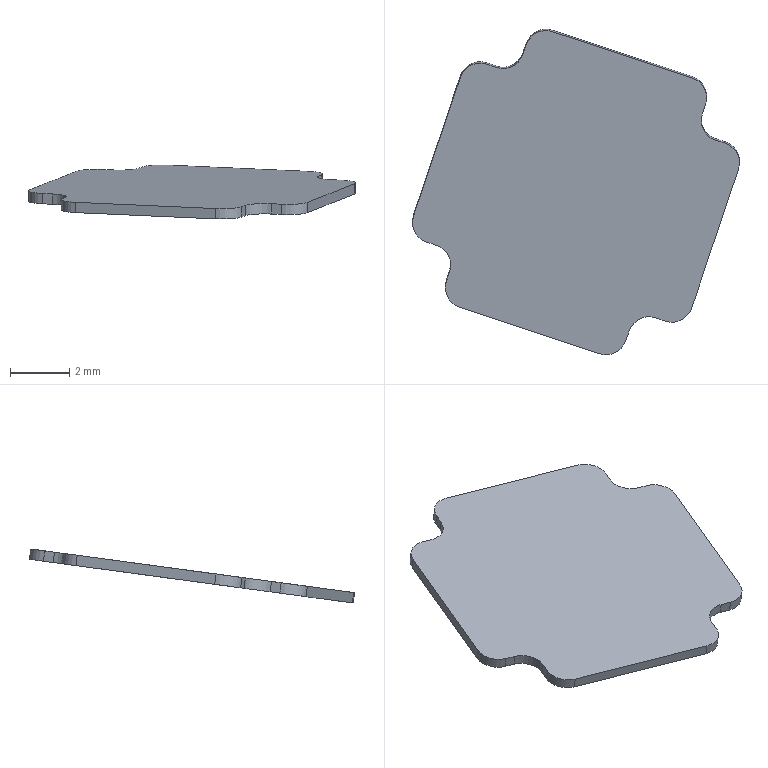Part | SolidWorks | features SplitBody 1 | 1 solid | 26 faces | box 11.072 x 11.019 x 1.829 mm | volume 30.173 mm3 | plane 14 | cylinder 12 | commonest cylinder face diameters 1.408 x12
STEP:
#1=CARTESIAN_POINT('',(543.22,367.896,-325.051));
#2=VERTEX_POINT('',#1);
#3=CARTESIAN_POINT('',(542.329,367.455,-325.11));
#4=VERTEX_POINT('',#3);
#5=CARTESIAN_POINT('',(542.997,367.234,-325.14));
#6=DIRECTION('',(0.,-0.1337,0.991));
#7=DIRECTION('',(0.317,0.9399,0.1268));
#8=AXIS2_PLACEMENT_3D('',#5,#6,#7);
#9=CIRCLE('',#8,0.704);
#10=EDGE_CURVE('',#2,#4,#9,.T.);
#11=ORIENTED_EDGE('',*,*,#10,.T.);
#12=CARTESIAN_POINT('',(542.329,367.408,-324.761));
#13=VERTEX_POINT('',#12);
#14=CARTESIAN_POINT('',(542.329,367.408,-324.761));
#15=DIRECTION('',(0.,0.1337,-0.991));
#16=VECTOR('',#15,1000.);
#17=LINE('',#14,#16);
#18=EDGE_CURVE('',#13,#4,#17,.T.);
#19=ORIENTED_EDGE('',*,*,#18,.F.);
#20=CARTESIAN_POINT('',(543.22,367.849,-324.702));
#21=VERTEX_POINT('',#20);
#22=CARTESIAN_POINT('',(542.997,367.187,-324.791));
#23=DIRECTION('',(0.,-0.1337,0.991));
#24=DIRECTION('',(0.317,0.9399,0.1268));
#25=AXIS2_PLACEMENT_3D('',#22,#23,#24);
#26=CIRCLE('',#25,0.704);
#27=EDGE_CURVE('',#21,#13,#26,.T.);
#28=ORIENTED_EDGE('',*,*,#27,.F.);
#29=CARTESIAN_POINT('',(543.22,367.849,-324.702));
#30=DIRECTION('',(0.,0.1337,-0.991));
#31=VECTOR('',#30,1000.);
#32=LINE('',#29,#31);
#33=EDGE_CURVE('',#21,#2,#32,.T.);
#34=ORIENTED_EDGE('',*,*,#33,.T.);
#35=EDGE_LOOP('',(#11,#19,#28,#34));
#36=FACE_OUTER_BOUND('',#35,.T.);
#37=CARTESIAN_POINT('',(542.997,367.187,-324.791));
#38=DIRECTION('',(0.,0.1337,-0.991));
#39=DIRECTION('',(0.317,0.9399,0.1268));
#40=AXIS2_PLACEMENT_3D('',#37,#38,#39);
#41=CYLINDRICAL_SURFACE('',#40,0.704);
#42=ADVANCED_FACE('',(#36),#41,.T.);
#43=CARTESIAN_POINT('',(542.217,367.125,-325.155));
#44=VERTEX_POINT('',#43);
#45=CARTESIAN_POINT('',(542.329,367.455,-325.11));
#46=DIRECTION('',(-0.317,-0.9399,-0.1268));
#47=VECTOR('',#46,1000.);
#48=LINE('',#45,#47);
#49=EDGE_CURVE('',#4,#44,#48,.T.);
#50=ORIENTED_EDGE('',*,*,#49,.T.);
#51=CARTESIAN_POINT('',(542.217,367.078,-324.806));
#52=VERTEX_POINT('',#51);
#53=CARTESIAN_POINT('',(542.217,367.078,-324.806));
#54=DIRECTION('',(0.,0.1337,-0.991));
#55=VECTOR('',#54,1000.);
#56=LINE('',#53,#55);
#57=EDGE_CURVE('',#52,#44,#56,.T.);
#58=ORIENTED_EDGE('',*,*,#57,.F.);
#59=CARTESIAN_POINT('',(542.329,367.408,-324.761));
#60=DIRECTION('',(-0.317,-0.9399,-0.1268));
#61=VECTOR('',#60,1000.);
#62=LINE('',#59,#61);
#63=EDGE_CURVE('',#13,#52,#62,.T.);
#64=ORIENTED_EDGE('',*,*,#63,.F.);
#65=ORIENTED_EDGE('',*,*,#18,.T.);
#66=EDGE_LOOP('',(#50,#58,#64,#65));
#67=FACE_OUTER_BOUND('',#66,.T.);
#68=CARTESIAN_POINT('',(542.329,367.408,-324.761));
#69=DIRECTION('',(0.9484,-0.3142,-0.04237));
#70=DIRECTION('',(0.,-0.1337,0.991));
#71=AXIS2_PLACEMENT_3D('',#68,#69,#70);
#72=PLANE('',#71);
#73=ADVANCED_FACE('',(#67),#72,.F.);
#74=CARTESIAN_POINT('',(541.326,366.684,-325.214));
#75=VERTEX_POINT('',#74);
#76=CARTESIAN_POINT('',(541.55,367.346,-325.125));
#77=DIRECTION('',(0.,0.1337,-0.991));
#78=DIRECTION('',(0.317,0.9399,0.1268));
#79=AXIS2_PLACEMENT_3D('',#76,#77,#78);
#80=CIRCLE('',#79,0.704);
#81=EDGE_CURVE('',#44,#75,#80,.T.);
#82=ORIENTED_EDGE('',*,*,#81,.T.);
#83=CARTESIAN_POINT('',(541.326,366.637,-324.865));
#84=VERTEX_POINT('',#83);
#85=CARTESIAN_POINT('',(541.326,366.637,-324.865));
#86=DIRECTION('',(0.,0.1337,-0.991));
#87=VECTOR('',#86,1000.);
#88=LINE('',#85,#87);
#89=EDGE_CURVE('',#84,#75,#88,.T.);
#90=ORIENTED_EDGE('',*,*,#89,.F.);
#91=CARTESIAN_POINT('',(541.55,367.299,-324.776));
#92=DIRECTION('',(0.,0.1337,-0.991));
#93=DIRECTION('',(0.317,0.9399,0.1268));
#94=AXIS2_PLACEMENT_3D('',#91,#92,#93);
#95=CIRCLE('',#94,0.704);
#96=EDGE_CURVE('',#52,#84,#95,.T.);
#97=ORIENTED_EDGE('',*,*,#96,.F.);
#98=ORIENTED_EDGE('',*,*,#57,.T.);
#99=EDGE_LOOP('',(#82,#90,#97,#98));
#100=FACE_OUTER_BOUND('',#99,.T.);
#101=CARTESIAN_POINT('',(541.55,367.299,-324.776));
#102=DIRECTION('',(0.,0.1337,-0.991));
#103=DIRECTION('',(0.317,0.9399,0.1268));
#104=AXIS2_PLACEMENT_3D('',#101,#102,#103);
#105=CYLINDRICAL_SURFACE('',#104,0.704);
#106=ADVANCED_FACE('',(#100),#105,.F.);
#107=CARTESIAN_POINT('',(540.993,366.795,-325.199));
#108=VERTEX_POINT('',#107);
#109=CARTESIAN_POINT('',(541.326,366.684,-325.214));
#110=DIRECTION('',(-0.9484,0.3142,0.04237));
#111=VECTOR('',#110,1000.);
#112=LINE('',#109,#111);
#113=EDGE_CURVE('',#75,#108,#112,.T.);
#114=ORIENTED_EDGE('',*,*,#113,.T.);
#115=CARTESIAN_POINT('',(540.993,366.748,-324.85));
#116=VERTEX_POINT('',#115);
#117=CARTESIAN_POINT('',(540.993,366.748,-324.85));
#118=DIRECTION('',(0.,0.1337,-0.991));
#119=VECTOR('',#118,1000.);
#120=LINE('',#117,#119);
#121=EDGE_CURVE('',#116,#108,#120,.T.);
#122=ORIENTED_EDGE('',*,*,#121,.F.);
#123=CARTESIAN_POINT('',(541.326,366.637,-324.865));
#124=DIRECTION('',(-0.9484,0.3142,0.04237));
#125=VECTOR('',#124,1000.);
#126=LINE('',#123,#125);
#127=EDGE_CURVE('',#84,#116,#126,.T.);
#128=ORIENTED_EDGE('',*,*,#127,.F.);
#129=ORIENTED_EDGE('',*,*,#89,.T.);
#130=EDGE_LOOP('',(#114,#122,#128,#129));
#131=FACE_OUTER_BOUND('',#130,.T.);
#132=CARTESIAN_POINT('',(541.326,366.637,-324.865));
#133=DIRECTION('',(-0.317,-0.9399,-0.1268));
#134=DIRECTION('',(0.,0.1337,-0.991));
#135=AXIS2_PLACEMENT_3D('',#132,#133,#134);
#136=PLANE('',#135);
#137=ADVANCED_FACE('',(#131),#136,.F.);
#138=CARTESIAN_POINT('',(540.102,366.354,-325.259));
#139=VERTEX_POINT('',#138);
#140=CARTESIAN_POINT('',(540.769,366.133,-325.288));
#141=DIRECTION('',(0.,-0.1337,0.991));
#142=DIRECTION('',(-0.317,-0.9399,-0.1268));
#143=AXIS2_PLACEMENT_3D('',#140,#141,#142);
#144=CIRCLE('',#143,0.704);
#145=EDGE_CURVE('',#108,#139,#144,.T.);
#146=ORIENTED_EDGE('',*,*,#145,.T.);
#147=CARTESIAN_POINT('',(540.102,366.307,-324.91));
#148=VERTEX_POINT('',#147);
#149=CARTESIAN_POINT('',(540.102,366.307,-324.91));
#150=DIRECTION('',(0.,0.1337,-0.991));
#151=VECTOR('',#150,1000.);
#152=LINE('',#149,#151);
#153=EDGE_CURVE('',#148,#139,#152,.T.);
#154=ORIENTED_EDGE('',*,*,#153,.F.);
#155=CARTESIAN_POINT('',(540.769,366.086,-324.94));
#156=DIRECTION('',(0.,-0.1337,0.991));
#157=DIRECTION('',(-0.317,-0.9399,-0.1268));
#158=AXIS2_PLACEMENT_3D('',#155,#156,#157);
#159=CIRCLE('',#158,0.704);
#160=EDGE_CURVE('',#116,#148,#159,.T.);
#161=ORIENTED_EDGE('',*,*,#160,.F.);
#162=ORIENTED_EDGE('',*,*,#121,.T.);
#163=EDGE_LOOP('',(#146,#154,#161,#162));
#164=FACE_OUTER_BOUND('',#163,.T.);
#165=CARTESIAN_POINT('',(540.769,366.086,-324.94));
#166=DIRECTION('',(0.,0.1337,-0.991));
#167=DIRECTION('',(0.317,0.9399,0.1268));
#168=AXIS2_PLACEMENT_3D('',#165,#166,#167);
#169=CYLINDRICAL_SURFACE('',#168,0.704);
#170=ADVANCED_FACE('',(#164),#169,.T.);
#171=CARTESIAN_POINT('',(538.517,361.656,-325.892));
#172=VERTEX_POINT('',#171);
#173=CARTESIAN_POINT('',(540.102,366.354,-325.259));
#174=DIRECTION('',(-0.317,-0.9399,-0.1268));
#175=VECTOR('',#174,1000.);
#176=LINE('',#173,#175);
#177=EDGE_CURVE('',#139,#172,#176,.T.);
#178=ORIENTED_EDGE('',*,*,#177,.T.);
#179=CARTESIAN_POINT('',(538.517,361.609,-325.543));
#180=VERTEX_POINT('',#179);
#181=CARTESIAN_POINT('',(538.517,361.609,-325.543));
#182=DIRECTION('',(0.,0.1337,-0.991));
#183=VECTOR('',#182,1000.);
#184=LINE('',#181,#183);
#185=EDGE_CURVE('',#180,#172,#184,.T.);
#186=ORIENTED_EDGE('',*,*,#185,.F.);
#187=CARTESIAN_POINT('',(540.102,366.307,-324.91));
#188=DIRECTION('',(-0.317,-0.9399,-0.1268));
#189=VECTOR('',#188,1000.);
#190=LINE('',#187,#189);
#191=EDGE_CURVE('',#148,#180,#190,.T.);
#192=ORIENTED_EDGE('',*,*,#191,.F.);
#193=ORIENTED_EDGE('',*,*,#153,.T.);
#194=EDGE_LOOP('',(#178,#186,#192,#193));
#195=FACE_OUTER_BOUND('',#194,.T.);
#196=CARTESIAN_POINT('',(540.102,366.307,-324.91));
#197=DIRECTION('',(0.9484,-0.3142,-0.04237));
#198=DIRECTION('',(0.,-0.1337,0.991));
#199=AXIS2_PLACEMENT_3D('',#196,#197,#198);
#200=PLANE('',#199);
#201=ADVANCED_FACE('',(#195),#200,.F.);
#202=CARTESIAN_POINT('',(538.962,360.773,-326.011));
#203=VERTEX_POINT('',#202);
#204=CARTESIAN_POINT('',(539.185,361.435,-325.922));
#205=DIRECTION('',(0.,-0.1337,0.991));
#206=DIRECTION('',(0.317,0.9399,0.1268));
#207=AXIS2_PLACEMENT_3D('',#204,#205,#206);
#208=CIRCLE('',#207,0.704);
#209=EDGE_CURVE('',#172,#203,#208,.T.);
#210=ORIENTED_EDGE('',*,*,#209,.T.);
#211=CARTESIAN_POINT('',(538.962,360.726,-325.662));
#212=VERTEX_POINT('',#211);
#213=CARTESIAN_POINT('',(538.962,360.726,-325.662));
#214=DIRECTION('',(0.,0.1337,-0.991));
#215=VECTOR('',#214,1000.);
#216=LINE('',#213,#215);
#217=EDGE_CURVE('',#212,#203,#216,.T.);
#218=ORIENTED_EDGE('',*,*,#217,.F.);
#219=CARTESIAN_POINT('',(539.185,361.388,-325.573));
#220=DIRECTION('',(0.,-0.1337,0.991));
#221=DIRECTION('',(0.317,0.9399,0.1268));
#222=AXIS2_PLACEMENT_3D('',#219,#220,#221);
#223=CIRCLE('',#222,0.704);
#224=EDGE_CURVE('',#180,#212,#223,.T.);
#225=ORIENTED_EDGE('',*,*,#224,.F.);
#226=ORIENTED_EDGE('',*,*,#185,.T.);
#227=EDGE_LOOP('',(#210,#218,#225,#226));
#228=FACE_OUTER_BOUND('',#227,.T.);
#229=CARTESIAN_POINT('',(539.185,361.388,-325.573));
#230=DIRECTION('',(0.,0.1337,-0.991));
#231=DIRECTION('',(0.317,0.9399,0.1268));
#232=AXIS2_PLACEMENT_3D('',#229,#230,#231);
#233=CYLINDRICAL_SURFACE('',#232,0.704);
#234=ADVANCED_FACE('',(#228),#233,.T.);
#235=CARTESIAN_POINT('',(539.296,360.663,-326.026));
#236=VERTEX_POINT('',#235);
#237=CARTESIAN_POINT('',(538.962,360.773,-326.011));
#238=DIRECTION('',(0.9484,-0.3142,-0.04237));
#239=VECTOR('',#238,1000.);
#240=LINE('',#237,#239);
#241=EDGE_CURVE('',#203,#236,#240,.T.);
#242=ORIENTED_EDGE('',*,*,#241,.T.);
#243=CARTESIAN_POINT('',(539.296,360.616,-325.677));
#244=VERTEX_POINT('',#243);
#245=CARTESIAN_POINT('',(539.296,360.616,-325.677));
#246=DIRECTION('',(0.,0.1337,-0.991));
#247=VECTOR('',#246,1000.);
#248=LINE('',#245,#247);
#249=EDGE_CURVE('',#244,#236,#248,.T.);
#250=ORIENTED_EDGE('',*,*,#249,.F.);
#251=CARTESIAN_POINT('',(538.962,360.726,-325.662));
#252=DIRECTION('',(0.9484,-0.3142,-0.04237));
#253=VECTOR('',#252,1000.);
#254=LINE('',#251,#253);
#255=EDGE_CURVE('',#212,#244,#254,.T.);
#256=ORIENTED_EDGE('',*,*,#255,.F.);
#257=ORIENTED_EDGE('',*,*,#217,.T.);
#258=EDGE_LOOP('',(#242,#250,#256,#257));
#259=FACE_OUTER_BOUND('',#258,.T.);
#260=CARTESIAN_POINT('',(538.962,360.726,-325.662));
#261=DIRECTION('',(0.317,0.9399,0.1268));
#262=DIRECTION('',(0.,-0.1337,0.991));
#263=AXIS2_PLACEMENT_3D('',#260,#261,#262);
#264=PLANE('',#263);
#265=ADVANCED_FACE('',(#259),#264,.F.);
#266=CARTESIAN_POINT('',(539.74,359.78,-326.145));
#267=VERTEX_POINT('',#266);
#268=CARTESIAN_POINT('',(539.072,360.001,-326.115));
#269=DIRECTION('',(0.,0.1337,-0.991));
#270=DIRECTION('',(0.317,0.9399,0.1268));
#271=AXIS2_PLACEMENT_3D('',#268,#269,#270);
#272=CIRCLE('',#271,0.704);
#273=EDGE_CURVE('',#236,#267,#272,.T.);
#274=ORIENTED_EDGE('',*,*,#273,.T.);
#275=CARTESIAN_POINT('',(539.74,359.733,-325.796));
#276=VERTEX_POINT('',#275);
#277=CARTESIAN_POINT('',(539.74,359.733,-325.796));
#278=DIRECTION('',(0.,0.1337,-0.991));
#279=VECTOR('',#278,1000.);
#280=LINE('',#277,#279);
#281=EDGE_CURVE('',#276,#267,#280,.T.);
#282=ORIENTED_EDGE('',*,*,#281,.F.);
#283=CARTESIAN_POINT('',(539.072,359.954,-325.767));
#284=DIRECTION('',(0.,0.1337,-0.991));
#285=DIRECTION('',(0.317,0.9399,0.1268));
#286=AXIS2_PLACEMENT_3D('',#283,#284,#285);
#287=CIRCLE('',#286,0.704);
#288=EDGE_CURVE('',#244,#276,#287,.T.);
#289=ORIENTED_EDGE('',*,*,#288,.F.);
#290=ORIENTED_EDGE('',*,*,#249,.T.);
#291=EDGE_LOOP('',(#274,#282,#289,#290));
#292=FACE_OUTER_BOUND('',#291,.T.);
#293=CARTESIAN_POINT('',(539.072,359.954,-325.767));
#294=DIRECTION('',(0.,0.1337,-0.991));
#295=DIRECTION('',(0.317,0.9399,0.1268));
#296=AXIS2_PLACEMENT_3D('',#293,#294,#295);
#297=CYLINDRICAL_SURFACE('',#296,0.704);
#298=ADVANCED_FACE('',(#292),#297,.F.);
#299=CARTESIAN_POINT('',(539.628,359.449,-326.19));
#300=VERTEX_POINT('',#299);
#301=CARTESIAN_POINT('',(539.74,359.78,-326.145));
#302=DIRECTION('',(-0.317,-0.9399,-0.1268));
#303=VECTOR('',#302,1000.);
#304=LINE('',#301,#303);
#305=EDGE_CURVE('',#267,#300,#304,.T.);
#306=ORIENTED_EDGE('',*,*,#305,.T.);
#307=CARTESIAN_POINT('',(539.628,359.402,-325.841));
#308=VERTEX_POINT('',#307);
#309=CARTESIAN_POINT('',(539.628,359.402,-325.841));
#310=DIRECTION('',(0.,0.1337,-0.991));
#311=VECTOR('',#310,1000.);
#312=LINE('',#309,#311);
#313=EDGE_CURVE('',#308,#300,#312,.T.);
#314=ORIENTED_EDGE('',*,*,#313,.F.);
#315=CARTESIAN_POINT('',(539.74,359.733,-325.796));
#316=DIRECTION('',(-0.317,-0.9399,-0.1268));
#317=VECTOR('',#316,1000.);
#318=LINE('',#315,#317);
#319=EDGE_CURVE('',#276,#308,#318,.T.);
#320=ORIENTED_EDGE('',*,*,#319,.F.);
#321=ORIENTED_EDGE('',*,*,#281,.T.);
#322=EDGE_LOOP('',(#306,#314,#320,#321));
#323=FACE_OUTER_BOUND('',#322,.T.);
#324=CARTESIAN_POINT('',(539.74,359.733,-325.796));
#325=DIRECTION('',(0.9484,-0.3142,-0.04237));
#326=DIRECTION('',(0.,-0.1337,0.991));
#327=AXIS2_PLACEMENT_3D('',#324,#325,#326);
#328=PLANE('',#327);
#329=ADVANCED_FACE('',(#323),#328,.F.);
#330=CARTESIAN_POINT('',(540.073,358.566,-326.309));
#331=VERTEX_POINT('',#330);
#332=CARTESIAN_POINT('',(540.296,359.228,-326.22));
#333=DIRECTION('',(0.,-0.1337,0.991));
#334=DIRECTION('',(-0.317,-0.9399,-0.1268));
#335=AXIS2_PLACEMENT_3D('',#332,#333,#334);
#336=CIRCLE('',#335,0.704);
#337=EDGE_CURVE('',#300,#331,#336,.T.);
#338=ORIENTED_EDGE('',*,*,#337,.T.);
#339=CARTESIAN_POINT('',(540.073,358.519,-325.96));
#340=VERTEX_POINT('',#339);
#341=CARTESIAN_POINT('',(540.073,358.519,-325.96));
#342=DIRECTION('',(0.,0.1337,-0.991));
#343=VECTOR('',#342,1000.);
#344=LINE('',#341,#343);
#345=EDGE_CURVE('',#340,#331,#344,.T.);
#346=ORIENTED_EDGE('',*,*,#345,.F.);
#347=CARTESIAN_POINT('',(540.296,359.181,-325.871));
#348=DIRECTION('',(0.,-0.1337,0.991));
#349=DIRECTION('',(-0.317,-0.9399,-0.1268));
#350=AXIS2_PLACEMENT_3D('',#347,#348,#349);
#351=CIRCLE('',#350,0.704);
#352=EDGE_CURVE('',#308,#340,#351,.T.);
#353=ORIENTED_EDGE('',*,*,#352,.F.);
#354=ORIENTED_EDGE('',*,*,#313,.T.);
#355=EDGE_LOOP('',(#338,#346,#353,#354));
#356=FACE_OUTER_BOUND('',#355,.T.);
#357=CARTESIAN_POINT('',(540.296,359.181,-325.871));
#358=DIRECTION('',(0.,0.1337,-0.991));
#359=DIRECTION('',(0.317,0.9399,0.1268));
#360=AXIS2_PLACEMENT_3D('',#357,#358,#359);
#361=CYLINDRICAL_SURFACE('',#360,0.704);
#362=ADVANCED_FACE('',(#356),#361,.T.);
#363=CARTESIAN_POINT('',(544.814,356.996,-326.521));
#364=VERTEX_POINT('',#363);
#365=CARTESIAN_POINT('',(540.073,358.566,-326.309));
#366=DIRECTION('',(0.9484,-0.3142,-0.04237));
#367=VECTOR('',#366,1000.);
#368=LINE('',#365,#367);
#369=EDGE_CURVE('',#331,#364,#368,.T.);
#370=ORIENTED_EDGE('',*,*,#369,.T.);
#371=CARTESIAN_POINT('',(544.814,356.949,-326.172));
#372=VERTEX_POINT('',#371);
#373=CARTESIAN_POINT('',(544.814,356.949,-326.172));
#374=DIRECTION('',(0.,0.1337,-0.991));
#375=VECTOR('',#374,1000.);
#376=LINE('',#373,#375);
#377=EDGE_CURVE('',#372,#364,#376,.T.);
#378=ORIENTED_EDGE('',*,*,#377,.F.);
#379=CARTESIAN_POINT('',(540.073,358.519,-325.96));
#380=DIRECTION('',(0.9484,-0.3142,-0.04237));
#381=VECTOR('',#380,1000.);
#382=LINE('',#379,#381);
#383=EDGE_CURVE('',#340,#372,#382,.T.);
#384=ORIENTED_EDGE('',*,*,#383,.F.);
#385=ORIENTED_EDGE('',*,*,#345,.T.);
#386=EDGE_LOOP('',(#370,#378,#384,#385));
#387=FACE_OUTER_BOUND('',#386,.T.);
#388=CARTESIAN_POINT('',(540.073,358.519,-325.96));
#389=DIRECTION('',(0.317,0.9399,0.1268));
#390=DIRECTION('',(-0.9484,0.3142,0.04237));
#391=AXIS2_PLACEMENT_3D('',#388,#389,#390);
#392=PLANE('',#391);
#393=ADVANCED_FACE('',(#387),#392,.F.);
#394=CARTESIAN_POINT('',(545.704,357.436,-326.461));
#395=VERTEX_POINT('',#394);
#396=CARTESIAN_POINT('',(545.037,357.657,-326.431));
#397=DIRECTION('',(0.,-0.1337,0.991));
#398=DIRECTION('',(0.317,0.9399,0.1268));
#399=AXIS2_PLACEMENT_3D('',#396,#397,#398);
#400=CIRCLE('',#399,0.704);
#401=EDGE_CURVE('',#364,#395,#400,.T.);
#402=ORIENTED_EDGE('',*,*,#401,.T.);
#403=CARTESIAN_POINT('',(545.704,357.389,-326.112));
#404=VERTEX_POINT('',#403);
#405=CARTESIAN_POINT('',(545.704,357.389,-326.112));
#406=DIRECTION('',(0.,0.1337,-0.991));
#407=VECTOR('',#406,1000.);
#408=LINE('',#405,#407);
#409=EDGE_CURVE('',#404,#395,#408,.T.);
#410=ORIENTED_EDGE('',*,*,#409,.F.);
#411=CARTESIAN_POINT('',(545.037,357.61,-326.083));
#412=DIRECTION('',(0.,-0.1337,0.991));
#413=DIRECTION('',(0.317,0.9399,0.1268));
#414=AXIS2_PLACEMENT_3D('',#411,#412,#413);
#415=CIRCLE('',#414,0.704);
#416=EDGE_CURVE('',#372,#404,#415,.T.);
#417=ORIENTED_EDGE('',*,*,#416,.F.);
#418=ORIENTED_EDGE('',*,*,#377,.T.);
#419=EDGE_LOOP('',(#402,#410,#417,#418));
#420=FACE_OUTER_BOUND('',#419,.T.);
#421=CARTESIAN_POINT('',(545.037,357.61,-326.083));
#422=DIRECTION('',(0.,0.1337,-0.991));
#423=DIRECTION('',(0.317,0.9399,0.1268));
#424=AXIS2_PLACEMENT_3D('',#421,#422,#423);
#425=CYLINDRICAL_SURFACE('',#424,0.704);
#426=ADVANCED_FACE('',(#420),#425,.T.);
#427=CARTESIAN_POINT('',(545.816,357.767,-326.417));
#428=VERTEX_POINT('',#427);
#429=CARTESIAN_POINT('',(545.816,357.767,-326.417));
#430=DIRECTION('',(0.317,0.9399,0.1268));
#431=VECTOR('',#430,1000.);
#432=LINE('',#429,#431);
#433=EDGE_CURVE('',#395,#428,#432,.T.);
#434=ORIENTED_EDGE('',*,*,#433,.T.);
#435=CARTESIAN_POINT('',(545.816,357.72,-326.068));
#436=VERTEX_POINT('',#435);
#437=CARTESIAN_POINT('',(545.816,357.72,-326.068));
#438=DIRECTION('',(0.,0.1337,-0.991));
#439=VECTOR('',#438,1000.);
#440=LINE('',#437,#439);
#441=EDGE_CURVE('',#436,#428,#440,.T.);
#442=ORIENTED_EDGE('',*,*,#441,.F.);
#443=CARTESIAN_POINT('',(545.816,357.72,-326.068));
#444=DIRECTION('',(0.317,0.9399,0.1268));
#445=VECTOR('',#444,1000.);
#446=LINE('',#443,#445);
#447=EDGE_CURVE('',#404,#436,#446,.T.);
#448=ORIENTED_EDGE('',*,*,#447,.F.);
#449=ORIENTED_EDGE('',*,*,#409,.T.);
#450=EDGE_LOOP('',(#434,#442,#448,#449));
#451=FACE_OUTER_BOUND('',#450,.T.);
#452=CARTESIAN_POINT('',(545.816,357.72,-326.068));
#453=DIRECTION('',(-0.9484,0.3142,0.04237));
#454=DIRECTION('',(0.,0.1337,-0.991));
#455=AXIS2_PLACEMENT_3D('',#452,#453,#454);
#456=PLANE('',#455);
#457=ADVANCED_FACE('',(#451),#456,.F.);
#458=CARTESIAN_POINT('',(546.707,358.208,-326.357));
#459=VERTEX_POINT('',#458);
#460=CARTESIAN_POINT('',(546.484,357.546,-326.446));
#461=DIRECTION('',(0.,0.1337,-0.991));
#462=DIRECTION('',(-0.317,-0.9399,-0.1268));
#463=AXIS2_PLACEMENT_3D('',#460,#461,#462);
#464=CIRCLE('',#463,0.704);
#465=EDGE_CURVE('',#428,#459,#464,.T.);
#466=ORIENTED_EDGE('',*,*,#465,.T.);
#467=CARTESIAN_POINT('',(546.707,358.161,-326.008));
#468=VERTEX_POINT('',#467);
#469=CARTESIAN_POINT('',(546.707,358.161,-326.008));
#470=DIRECTION('',(0.,0.1337,-0.991));
#471=VECTOR('',#470,1000.);
#472=LINE('',#469,#471);
#473=EDGE_CURVE('',#468,#459,#472,.T.);
#474=ORIENTED_EDGE('',*,*,#473,.F.);
#475=CARTESIAN_POINT('',(546.484,357.499,-326.098));
#476=DIRECTION('',(0.,0.1337,-0.991));
#477=DIRECTION('',(-0.317,-0.9399,-0.1268));
#478=AXIS2_PLACEMENT_3D('',#475,#476,#477);
#479=CIRCLE('',#478,0.704);
#480=EDGE_CURVE('',#436,#468,#479,.T.);
#481=ORIENTED_EDGE('',*,*,#480,.F.);
#482=ORIENTED_EDGE('',*,*,#441,.T.);
#483=EDGE_LOOP('',(#466,#474,#481,#482));
#484=FACE_OUTER_BOUND('',#483,.T.);
#485=CARTESIAN_POINT('',(546.484,357.499,-326.098));
#486=DIRECTION('',(0.,0.1337,-0.991));
#487=DIRECTION('',(0.317,0.9399,0.1268));
#488=AXIS2_PLACEMENT_3D('',#485,#486,#487);
#489=CYLINDRICAL_SURFACE('',#488,0.704);
#490=ADVANCED_FACE('',(#484),#489,.F.);
#491=CARTESIAN_POINT('',(547.041,358.097,-326.372));
#492=VERTEX_POINT('',#491);
#493=CARTESIAN_POINT('',(547.041,358.097,-326.372));
#494=DIRECTION('',(0.9484,-0.3142,-0.04237));
#495=VECTOR('',#494,1000.);
#496=LINE('',#493,#495);
#497=EDGE_CURVE('',#459,#492,#496,.T.);
#498=ORIENTED_EDGE('',*,*,#497,.T.);
#499=CARTESIAN_POINT('',(547.041,358.05,-326.023));
#500=VERTEX_POINT('',#499);
#501=CARTESIAN_POINT('',(547.041,358.05,-326.023));
#502=DIRECTION('',(0.,0.1337,-0.991));
#503=VECTOR('',#502,1000.);
#504=LINE('',#501,#503);
#505=EDGE_CURVE('',#500,#492,#504,.T.);
#506=ORIENTED_EDGE('',*,*,#505,.F.);
#507=CARTESIAN_POINT('',(547.041,358.05,-326.023));
#508=DIRECTION('',(0.9484,-0.3142,-0.04237));
#509=VECTOR('',#508,1000.);
#510=LINE('',#507,#509);
#511=EDGE_CURVE('',#468,#500,#510,.T.);
#512=ORIENTED_EDGE('',*,*,#511,.F.);
#513=ORIENTED_EDGE('',*,*,#473,.T.);
#514=EDGE_LOOP('',(#498,#506,#512,#513));
#515=FACE_OUTER_BOUND('',#514,.T.);
#516=CARTESIAN_POINT('',(547.041,358.05,-326.023));
#517=DIRECTION('',(0.317,0.9399,0.1268));
#518=DIRECTION('',(0.,-0.1337,0.991));
#519=AXIS2_PLACEMENT_3D('',#516,#517,#518);
#520=PLANE('',#519);
#521=ADVANCED_FACE('',(#515),#520,.F.);
#522=CARTESIAN_POINT('',(547.932,358.538,-326.313));
#523=VERTEX_POINT('',#522);
#524=CARTESIAN_POINT('',(547.264,358.759,-326.283));
#525=DIRECTION('',(0.,-0.1337,0.991));
#526=DIRECTION('',(-0.317,-0.9399,-0.1268));
#527=AXIS2_PLACEMENT_3D('',#524,#525,#526);
#528=CIRCLE('',#527,0.704);
#529=EDGE_CURVE('',#492,#523,#528,.T.);
#530=ORIENTED_EDGE('',*,*,#529,.T.);
#531=CARTESIAN_POINT('',(547.932,358.491,-325.964));
#532=VERTEX_POINT('',#531);
#533=CARTESIAN_POINT('',(547.932,358.491,-325.964));
#534=DIRECTION('',(0.,0.1337,-0.991));
#535=VECTOR('',#534,1000.);
#536=LINE('',#533,#535);
#537=EDGE_CURVE('',#532,#523,#536,.T.);
#538=ORIENTED_EDGE('',*,*,#537,.F.);
#539=CARTESIAN_POINT('',(547.264,358.712,-325.934));
#540=DIRECTION('',(0.,-0.1337,0.991));
#541=DIRECTION('',(-0.317,-0.9399,-0.1268));
#542=AXIS2_PLACEMENT_3D('',#539,#540,#541);
#543=CIRCLE('',#542,0.704);
#544=EDGE_CURVE('',#500,#532,#543,.T.);
#545=ORIENTED_EDGE('',*,*,#544,.F.);
#546=ORIENTED_EDGE('',*,*,#505,.T.);
#547=EDGE_LOOP('',(#530,#538,#545,#546));
#548=FACE_OUTER_BOUND('',#547,.T.);
#549=CARTESIAN_POINT('',(547.264,358.712,-325.934));
#550=DIRECTION('',(0.,0.1337,-0.991));
#551=DIRECTION('',(0.317,0.9399,0.1268));
#552=AXIS2_PLACEMENT_3D('',#549,#550,#551);
#553=CYLINDRICAL_SURFACE('',#552,0.704);
#554=ADVANCED_FACE('',(#548),#553,.T.);
#555=CARTESIAN_POINT('',(549.516,363.236,-325.679));
#556=VERTEX_POINT('',#555);
#557=CARTESIAN_POINT('',(549.516,363.236,-325.679));
#558=DIRECTION('',(0.317,0.9399,0.1268));
#559=VECTOR('',#558,1000.);
#560=LINE('',#557,#559);
#561=EDGE_CURVE('',#523,#556,#560,.T.);
#562=ORIENTED_EDGE('',*,*,#561,.T.);
#563=CARTESIAN_POINT('',(549.516,363.189,-325.33));
#564=VERTEX_POINT('',#563);
#565=CARTESIAN_POINT('',(549.516,363.189,-325.33));
#566=DIRECTION('',(0.,0.1337,-0.991));
#567=VECTOR('',#566,1000.);
#568=LINE('',#565,#567);
#569=EDGE_CURVE('',#564,#556,#568,.T.);
#570=ORIENTED_EDGE('',*,*,#569,.F.);
#571=CARTESIAN_POINT('',(549.516,363.189,-325.33));
#572=DIRECTION('',(0.317,0.9399,0.1268));
#573=VECTOR('',#572,1000.);
#574=LINE('',#571,#573);
#575=EDGE_CURVE('',#532,#564,#574,.T.);
#576=ORIENTED_EDGE('',*,*,#575,.F.);
#577=ORIENTED_EDGE('',*,*,#537,.T.);
#578=EDGE_LOOP('',(#562,#570,#576,#577));
#579=FACE_OUTER_BOUND('',#578,.T.);
#580=CARTESIAN_POINT('',(549.516,363.189,-325.33));
#581=DIRECTION('',(-0.9484,0.3142,0.04237));
#582=DIRECTION('',(0.,0.1337,-0.991));
#583=AXIS2_PLACEMENT_3D('',#580,#581,#582);
#584=PLANE('',#583);
#585=ADVANCED_FACE('',(#579),#584,.F.);
#586=CARTESIAN_POINT('',(549.072,364.119,-325.56));
#587=VERTEX_POINT('',#586);
#588=CARTESIAN_POINT('',(548.848,363.457,-325.649));
#589=DIRECTION('',(0.,-0.1337,0.991));
#590=DIRECTION('',(0.317,0.9399,0.1268));
#591=AXIS2_PLACEMENT_3D('',#588,#589,#590);
#592=CIRCLE('',#591,0.704);
#593=EDGE_CURVE('',#556,#587,#592,.T.);
#594=ORIENTED_EDGE('',*,*,#593,.T.);
#595=CARTESIAN_POINT('',(549.072,364.071,-325.211));
#596=VERTEX_POINT('',#595);
#597=CARTESIAN_POINT('',(549.072,364.071,-325.211));
#598=DIRECTION('',(0.,0.1337,-0.991));
#599=VECTOR('',#598,1000.);
#600=LINE('',#597,#599);
#601=EDGE_CURVE('',#596,#587,#600,.T.);
#602=ORIENTED_EDGE('',*,*,#601,.F.);
#603=CARTESIAN_POINT('',(548.848,363.41,-325.3));
#604=DIRECTION('',(0.,-0.1337,0.991));
#605=DIRECTION('',(0.317,0.9399,0.1268));
#606=AXIS2_PLACEMENT_3D('',#603,#604,#605);
#607=CIRCLE('',#606,0.704);
#608=EDGE_CURVE('',#564,#596,#607,.T.);
#609=ORIENTED_EDGE('',*,*,#608,.F.);
#610=ORIENTED_EDGE('',*,*,#569,.T.);
#611=EDGE_LOOP('',(#594,#602,#609,#610));
#612=FACE_OUTER_BOUND('',#611,.T.);
#613=CARTESIAN_POINT('',(548.848,363.41,-325.3));
#614=DIRECTION('',(0.,0.1337,-0.991));
#615=DIRECTION('',(0.317,0.9399,0.1268));
#616=AXIS2_PLACEMENT_3D('',#613,#614,#615);
#617=CYLINDRICAL_SURFACE('',#616,0.704);
#618=ADVANCED_FACE('',(#612),#617,.T.);
#619=CARTESIAN_POINT('',(548.738,364.229,-325.545));
#620=VERTEX_POINT('',#619);
#621=CARTESIAN_POINT('',(549.072,364.119,-325.56));
#622=DIRECTION('',(-0.9484,0.3142,0.04237));
#623=VECTOR('',#622,1000.);
#624=LINE('',#621,#623);
#625=EDGE_CURVE('',#587,#620,#624,.T.);
#626=ORIENTED_EDGE('',*,*,#625,.T.);
#627=CARTESIAN_POINT('',(548.738,364.182,-325.196));
#628=VERTEX_POINT('',#627);
#629=CARTESIAN_POINT('',(548.738,364.182,-325.196));
#630=DIRECTION('',(0.,0.1337,-0.991));
#631=VECTOR('',#630,1000.);
#632=LINE('',#629,#631);
#633=EDGE_CURVE('',#628,#620,#632,.T.);
#634=ORIENTED_EDGE('',*,*,#633,.F.);
#635=CARTESIAN_POINT('',(549.072,364.071,-325.211));
#636=DIRECTION('',(-0.9484,0.3142,0.04237));
#637=VECTOR('',#636,1000.);
#638=LINE('',#635,#637);
#639=EDGE_CURVE('',#596,#628,#638,.T.);
#640=ORIENTED_EDGE('',*,*,#639,.F.);
#641=ORIENTED_EDGE('',*,*,#601,.T.);
#642=EDGE_LOOP('',(#626,#634,#640,#641));
#643=FACE_OUTER_BOUND('',#642,.T.);
#644=CARTESIAN_POINT('',(549.072,364.071,-325.211));
#645=DIRECTION('',(-0.317,-0.9399,-0.1268));
#646=DIRECTION('',(0.,0.1337,-0.991));
#647=AXIS2_PLACEMENT_3D('',#644,#645,#646);
#648=PLANE('',#647);
#649=ADVANCED_FACE('',(#643),#648,.F.);
#650=CARTESIAN_POINT('',(548.293,365.112,-325.426));
#651=VERTEX_POINT('',#650);
#652=CARTESIAN_POINT('',(548.961,364.891,-325.456));
#653=DIRECTION('',(0.,0.1337,-0.991));
#654=DIRECTION('',(0.317,0.9399,0.1268));
#655=AXIS2_PLACEMENT_3D('',#652,#653,#654);
#656=CIRCLE('',#655,0.704);
#657=EDGE_CURVE('',#620,#651,#656,.T.);
#658=ORIENTED_EDGE('',*,*,#657,.T.);
#659=CARTESIAN_POINT('',(548.293,365.065,-325.077));
#660=VERTEX_POINT('',#659);
#661=CARTESIAN_POINT('',(548.293,365.065,-325.077));
#662=DIRECTION('',(0.,0.1337,-0.991));
#663=VECTOR('',#662,1000.);
#664=LINE('',#661,#663);
#665=EDGE_CURVE('',#660,#651,#664,.T.);
#666=ORIENTED_EDGE('',*,*,#665,.F.);
#667=CARTESIAN_POINT('',(548.961,364.844,-325.107));
#668=DIRECTION('',(0.,0.1337,-0.991));
#669=DIRECTION('',(0.317,0.9399,0.1268));
#670=AXIS2_PLACEMENT_3D('',#667,#668,#669);
#671=CIRCLE('',#670,0.704);
#672=EDGE_CURVE('',#628,#660,#671,.T.);
#673=ORIENTED_EDGE('',*,*,#672,.F.);
#674=ORIENTED_EDGE('',*,*,#633,.T.);
#675=EDGE_LOOP('',(#658,#666,#673,#674));
#676=FACE_OUTER_BOUND('',#675,.T.);
#677=CARTESIAN_POINT('',(548.961,364.844,-325.107));
#678=DIRECTION('',(0.,0.1337,-0.991));
#679=DIRECTION('',(0.317,0.9399,0.1268));
#680=AXIS2_PLACEMENT_3D('',#677,#678,#679);
#681=CYLINDRICAL_SURFACE('',#680,0.704);
#682=ADVANCED_FACE('',(#676),#681,.F.);
#683=CARTESIAN_POINT('',(548.405,365.443,-325.381));
#684=VERTEX_POINT('',#683);
#685=CARTESIAN_POINT('',(548.293,365.112,-325.426));
#686=DIRECTION('',(0.317,0.9399,0.1268));
#687=VECTOR('',#686,1000.);
#688=LINE('',#685,#687);
#689=EDGE_CURVE('',#651,#684,#688,.T.);
#690=ORIENTED_EDGE('',*,*,#689,.T.);
#691=CARTESIAN_POINT('',(548.405,365.396,-325.033));
#692=VERTEX_POINT('',#691);
#693=CARTESIAN_POINT('',(548.405,365.396,-325.033));
#694=DIRECTION('',(0.,0.1337,-0.991));
#695=VECTOR('',#694,1000.);
#696=LINE('',#693,#695);
#697=EDGE_CURVE('',#692,#684,#696,.T.);
#698=ORIENTED_EDGE('',*,*,#697,.F.);
#699=CARTESIAN_POINT('',(548.293,365.065,-325.077));
#700=DIRECTION('',(0.317,0.9399,0.1268));
#701=VECTOR('',#700,1000.);
#702=LINE('',#699,#701);
#703=EDGE_CURVE('',#660,#692,#702,.T.);
#704=ORIENTED_EDGE('',*,*,#703,.F.);
#705=ORIENTED_EDGE('',*,*,#665,.T.);
#706=EDGE_LOOP('',(#690,#698,#704,#705));
#707=FACE_OUTER_BOUND('',#706,.T.);
#708=CARTESIAN_POINT('',(548.293,365.065,-325.077));
#709=DIRECTION('',(-0.9484,0.3142,0.04237));
#710=DIRECTION('',(0.,0.1337,-0.991));
#711=AXIS2_PLACEMENT_3D('',#708,#709,#710);
#712=PLANE('',#711);
#713=ADVANCED_FACE('',(#707),#712,.F.);
#714=CARTESIAN_POINT('',(547.96,366.326,-325.262));
#715=VERTEX_POINT('',#714);
#716=CARTESIAN_POINT('',(547.737,365.664,-325.352));
#717=DIRECTION('',(0.,-0.1337,0.991));
#718=DIRECTION('',(-0.317,-0.9399,-0.1268));
#719=AXIS2_PLACEMENT_3D('',#716,#717,#718);
#720=CIRCLE('',#719,0.704);
#721=EDGE_CURVE('',#684,#715,#720,.T.);
#722=ORIENTED_EDGE('',*,*,#721,.T.);
#723=CARTESIAN_POINT('',(547.96,366.279,-324.914));
#724=VERTEX_POINT('',#723);
#725=CARTESIAN_POINT('',(547.96,366.279,-324.914));
#726=DIRECTION('',(0.,0.1337,-0.991));
#727=VECTOR('',#726,1000.);
#728=LINE('',#725,#727);
#729=EDGE_CURVE('',#724,#715,#728,.T.);
#730=ORIENTED_EDGE('',*,*,#729,.F.);
#731=CARTESIAN_POINT('',(547.737,365.617,-325.003));
#732=DIRECTION('',(0.,-0.1337,0.991));
#733=DIRECTION('',(-0.317,-0.9399,-0.1268));
#734=AXIS2_PLACEMENT_3D('',#731,#732,#733);
#735=CIRCLE('',#734,0.704);
#736=EDGE_CURVE('',#692,#724,#735,.T.);
#737=ORIENTED_EDGE('',*,*,#736,.F.);
#738=ORIENTED_EDGE('',*,*,#697,.T.);
#739=EDGE_LOOP('',(#722,#730,#737,#738));
#740=FACE_OUTER_BOUND('',#739,.T.);
#741=CARTESIAN_POINT('',(547.737,365.617,-325.003));
#742=DIRECTION('',(0.,0.1337,-0.991));
#743=DIRECTION('',(0.317,0.9399,0.1268));
#744=AXIS2_PLACEMENT_3D('',#741,#742,#743);
#745=CYLINDRICAL_SURFACE('',#744,0.704);
#746=ADVANCED_FACE('',(#740),#745,.T.);
#747=CARTESIAN_POINT('',(543.22,367.896,-325.051));
#748=DIRECTION('',(-0.9484,0.3142,0.04237));
#749=VECTOR('',#748,1000.);
#750=LINE('',#747,#749);
#751=EDGE_CURVE('',#715,#2,#750,.T.);
#752=ORIENTED_EDGE('',*,*,#751,.T.);
#753=ORIENTED_EDGE('',*,*,#33,.F.);
#754=CARTESIAN_POINT('',(543.22,367.849,-324.702));
#755=DIRECTION('',(-0.9484,0.3142,0.04237));
#756=VECTOR('',#755,1000.);
#757=LINE('',#754,#756);
#758=EDGE_CURVE('',#724,#21,#757,.T.);
#759=ORIENTED_EDGE('',*,*,#758,.F.);
#760=ORIENTED_EDGE('',*,*,#729,.T.);
#761=EDGE_LOOP('',(#752,#753,#759,#760));
#762=FACE_OUTER_BOUND('',#761,.T.);
#763=CARTESIAN_POINT('',(543.22,367.849,-324.702));
#764=DIRECTION('',(-0.317,-0.9399,-0.1268));
#765=DIRECTION('',(0.,0.1337,-0.991));
#766=AXIS2_PLACEMENT_3D('',#763,#764,#765);
#767=PLANE('',#766);
#768=ADVANCED_FACE('',(#762),#767,.F.);
#769=ORIENTED_EDGE('',*,*,#27,.T.);
#770=ORIENTED_EDGE('',*,*,#63,.T.);
#771=ORIENTED_EDGE('',*,*,#96,.T.);
#772=ORIENTED_EDGE('',*,*,#127,.T.);
#773=ORIENTED_EDGE('',*,*,#160,.T.);
#774=ORIENTED_EDGE('',*,*,#191,.T.);
#775=ORIENTED_EDGE('',*,*,#224,.T.);
#776=ORIENTED_EDGE('',*,*,#255,.T.);
#777=ORIENTED_EDGE('',*,*,#288,.T.);
#778=ORIENTED_EDGE('',*,*,#319,.T.);
#779=ORIENTED_EDGE('',*,*,#352,.T.);
#780=ORIENTED_EDGE('',*,*,#383,.T.);
#781=ORIENTED_EDGE('',*,*,#416,.T.);
#782=ORIENTED_EDGE('',*,*,#447,.T.);
#783=ORIENTED_EDGE('',*,*,#480,.T.);
#784=ORIENTED_EDGE('',*,*,#511,.T.);
#785=ORIENTED_EDGE('',*,*,#544,.T.);
#786=ORIENTED_EDGE('',*,*,#575,.T.);
#787=ORIENTED_EDGE('',*,*,#608,.T.);
#788=ORIENTED_EDGE('',*,*,#639,.T.);
#789=ORIENTED_EDGE('',*,*,#672,.T.);
#790=ORIENTED_EDGE('',*,*,#703,.T.);
#791=ORIENTED_EDGE('',*,*,#736,.T.);
#792=ORIENTED_EDGE('',*,*,#758,.T.);
#793=EDGE_LOOP('',(#769,#770,#771,#772,#773,#774,#775,#776,#777,#778,#779,#780,#781,#782,#783,#784,#785,#786,#787,#788,#789,#790,#791,#792));
#794=FACE_OUTER_BOUND('',#793,.T.);
#795=CARTESIAN_POINT('',(542.997,367.187,-324.791));
#796=DIRECTION('',(0.,0.1337,-0.991));
#797=DIRECTION('',(0.317,0.9399,0.1268));
#798=AXIS2_PLACEMENT_3D('',#795,#796,#797);
#799=PLANE('',#798);
#800=ADVANCED_FACE('',(#794),#799,.F.);
#801=ORIENTED_EDGE('',*,*,#10,.F.);
#802=ORIENTED_EDGE('',*,*,#751,.F.);
#803=ORIENTED_EDGE('',*,*,#721,.F.);
#804=ORIENTED_EDGE('',*,*,#689,.F.);
#805=ORIENTED_EDGE('',*,*,#657,.F.);
#806=ORIENTED_EDGE('',*,*,#625,.F.);
#807=ORIENTED_EDGE('',*,*,#593,.F.);
#808=ORIENTED_EDGE('',*,*,#561,.F.);
#809=ORIENTED_EDGE('',*,*,#529,.F.);
#810=ORIENTED_EDGE('',*,*,#497,.F.);
#811=ORIENTED_EDGE('',*,*,#465,.F.);
#812=ORIENTED_EDGE('',*,*,#433,.F.);
#813=ORIENTED_EDGE('',*,*,#401,.F.);
#814=ORIENTED_EDGE('',*,*,#369,.F.);
#815=ORIENTED_EDGE('',*,*,#337,.F.);
#816=ORIENTED_EDGE('',*,*,#305,.F.);
#817=ORIENTED_EDGE('',*,*,#273,.F.);
#818=ORIENTED_EDGE('',*,*,#241,.F.);
#819=ORIENTED_EDGE('',*,*,#209,.F.);
#820=ORIENTED_EDGE('',*,*,#177,.F.);
#821=ORIENTED_EDGE('',*,*,#145,.F.);
#822=ORIENTED_EDGE('',*,*,#113,.F.);
#823=ORIENTED_EDGE('',*,*,#81,.F.);
#824=ORIENTED_EDGE('',*,*,#49,.F.);
#825=EDGE_LOOP('',(#801,#802,#803,#804,#805,#806,#807,#808,#809,#810,#811,#812,#813,#814,#815,#816,#817,#818,#819,#820,#821,#822,#823,#824));
#826=FACE_OUTER_BOUND('',#825,.T.);
#827=CARTESIAN_POINT('',(542.997,367.234,-325.14));
#828=DIRECTION('',(0.,0.1337,-0.991));
#829=DIRECTION('',(0.317,0.9399,0.1268));
#830=AXIS2_PLACEMENT_3D('',#827,#828,#829);
#831=PLANE('',#830);
#832=ADVANCED_FACE('',(#826),#831,.T.);
#833=CLOSED_SHELL('',(#42,#73,#106,#137,#170,#201,#234,#265,#298,#329,#362,#393,#426,#457,#490,#521,#554,#585,#618,#649,#682,#713,#746,#768,#800,#832));
#834=MANIFOLD_SOLID_BREP('',#833);
#835=CARTESIAN_POINT('',(0.,0.,0.));
#836=DIRECTION('',(0.,0.,1.));
#837=DIRECTION('',(1.,0.,0.));
#838=AXIS2_PLACEMENT_3D('',#835,#836,#837);
#839=(LENGTH_UNIT()NAMED_UNIT(*)SI_UNIT(.MILLI.,.METRE.));
#840=UNCERTAINTY_MEASURE_WITH_UNIT(LENGTH_MEASURE(0.00001),#839,'','');
#841=(NAMED_UNIT(*)PLANE_ANGLE_UNIT()SI_UNIT($,.RADIAN.));
#842=(NAMED_UNIT(*)SI_UNIT($,.STERADIAN.)SOLID_ANGLE_UNIT());
#843=(GEOMETRIC_REPRESENTATION_CONTEXT(3)GLOBAL_UNCERTAINTY_ASSIGNED_CONTEXT((#840))GLOBAL_UNIT_ASSIGNED_CONTEXT((#839,#841,#842))REPRESENTATION_CONTEXT('',''));
#844=ADVANCED_BREP_SHAPE_REPRESENTATION('',(#834,#838),#843);